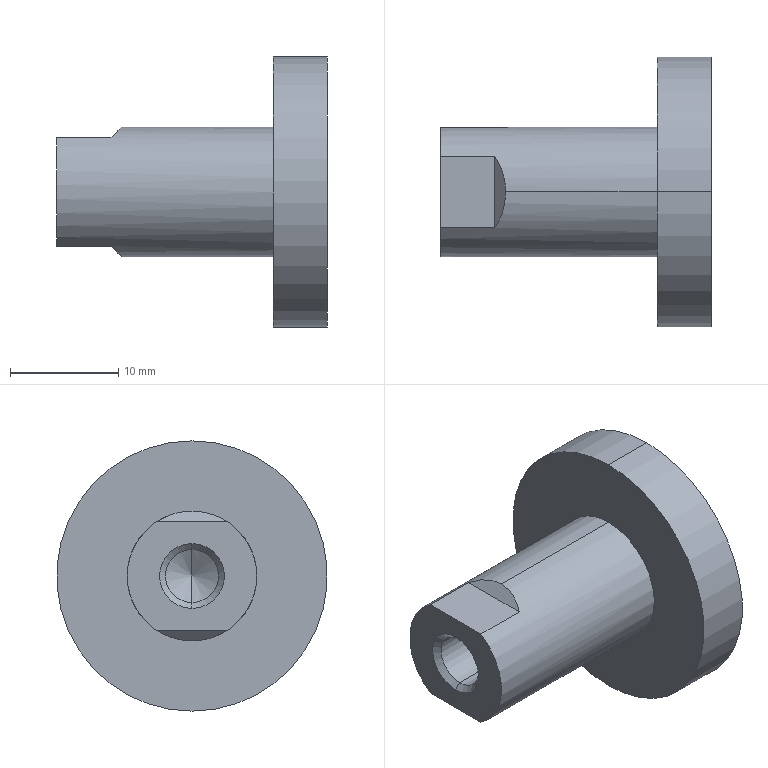Part | STEP file | 2_9 | 1 solid | 17 faces | box 25 x 25 x 25 mm | volume 4428 mm3 | plane 7 | cylinder 6 | cone 4 | commonest cylinder face diameters 4.917 x2 12 x2 25 x2
STEP:
#1=CARTESIAN_POINT('',(0.,0.,0.));
#2=DIRECTION('',(0.,0.,1.));
#3=DIRECTION('',(1.,0.,0.));
#4=AXIS2_PLACEMENT_3D('',#1,#2,#3);
#5=CARTESIAN_POINT('',(15.,0.,-12.5));
#6=VERTEX_POINT('',#5);
#7=CARTESIAN_POINT('',(15.,0.,12.5));
#8=VERTEX_POINT('',#7);
#9=CARTESIAN_POINT('',(15.,0.,0.));
#10=DIRECTION('',(1.,0.,0.));
#11=DIRECTION('',(0.,0.,-1.));
#12=AXIS2_PLACEMENT_3D('',#9,#10,#11);
#13=CIRCLE('',#12,12.5);
#14=CARTESIAN_POINT('',(17.5,0.,0.));
#15=DIRECTION('',(1.,0.,0.));
#16=DIRECTION('',(0.,0.,-1.));
#17=AXIS2_PLACEMENT_3D('',#14,#15,#16);
#18=CYLINDRICAL_SURFACE('',#17,12.5);
#19=CARTESIAN_POINT('',(0.,-2.5));
#20=DIRECTION('',(1.,0.));
#21=VECTOR('',#20,1.);
#22=LINE('',#19,#21);
#23=(GEOMETRIC_REPRESENTATION_CONTEXT(2)PARAMETRIC_REPRESENTATION_CONTEXT()REPRESENTATION_CONTEXT('',''));
#24=DEFINITIONAL_REPRESENTATION('',(#22),#23);
#25=PCURVE('',#18,#24);
#26=CARTESIAN_POINT('',(15.,9.25,0.));
#27=DIRECTION('',(-1.,0.,0.));
#28=DIRECTION('',(0.,0.,1.));
#29=AXIS2_PLACEMENT_3D('',#26,#27,#28);
#30=PLANE('',#29);
#31=CARTESIAN_POINT('',(-12.5,-9.25));
#32=CARTESIAN_POINT('',(-12.5,12.401));
#33=CARTESIAN_POINT('',(6.25,1.575));
#34=CARTESIAN_POINT('',(25.,-9.25));
#35=CARTESIAN_POINT('',(6.25,-20.075));
#36=CARTESIAN_POINT('',(-12.5,-30.901));
#37=CARTESIAN_POINT('',(-12.5,-9.25));
#38=(BOUNDED_CURVE()B_SPLINE_CURVE(2,(#31,#32,#33,#34,#35,#36,#37),.UNSPECIFIED.,.T.,.F.)B_SPLINE_CURVE_WITH_KNOTS((1,2,2,2,2,1),(-2.094,0.,2.094,4.189,6.283,8.378),.UNSPECIFIED.)CURVE()GEOMETRIC_REPRESENTATION_ITEM()RATIONAL_B_SPLINE_CURVE((1.,0.5,1.,0.5,1.,0.5,1.))REPRESENTATION_ITEM(''));
#39=(GEOMETRIC_REPRESENTATION_CONTEXT(2)PARAMETRIC_REPRESENTATION_CONTEXT()REPRESENTATION_CONTEXT('',''));
#40=DEFINITIONAL_REPRESENTATION('',(#38),#39);
#41=PCURVE('',#30,#40);
#42=SURFACE_CURVE('',#13,(#25,#41),.PCURVE_S1.);
#43=EDGE_CURVE('',#6,#8,#42,.T.);
#44=ORIENTED_EDGE('',*,*,#43,.T.);
#45=CARTESIAN_POINT('',(20.,0.,12.5));
#46=VERTEX_POINT('',#45);
#47=CARTESIAN_POINT('',(17.5,0.,12.5));
#48=DIRECTION('',(1.,0.,0.));
#49=VECTOR('',#48,1.);
#50=LINE('',#47,#49);
#51=CARTESIAN_POINT('',(3.142,0.));
#52=DIRECTION('',(0.,1.));
#53=VECTOR('',#52,1.);
#54=LINE('',#51,#53);
#55=(GEOMETRIC_REPRESENTATION_CONTEXT(2)PARAMETRIC_REPRESENTATION_CONTEXT()REPRESENTATION_CONTEXT('',''));
#56=DEFINITIONAL_REPRESENTATION('',(#54),#55);
#57=PCURVE('',#18,#56);
#58=CARTESIAN_POINT('',(17.5,0.,0.));
#59=DIRECTION('',(1.,0.,0.));
#60=DIRECTION('',(0.,0.,-1.));
#61=AXIS2_PLACEMENT_3D('',#58,#59,#60);
#62=CYLINDRICAL_SURFACE('',#61,12.5);
#63=CARTESIAN_POINT('',(3.142,0.));
#64=DIRECTION('',(0.,1.));
#65=VECTOR('',#64,1.);
#66=LINE('',#63,#65);
#67=(GEOMETRIC_REPRESENTATION_CONTEXT(2)PARAMETRIC_REPRESENTATION_CONTEXT()REPRESENTATION_CONTEXT('',''));
#68=DEFINITIONAL_REPRESENTATION('',(#66),#67);
#69=PCURVE('',#62,#68);
#70=SURFACE_CURVE('',#50,(#57,#69),.PCURVE_S1.);
#71=EDGE_CURVE('',#8,#46,#70,.T.);
#72=ORIENTED_EDGE('',*,*,#71,.T.);
#73=CARTESIAN_POINT('',(20.,0.,-12.5));
#74=VERTEX_POINT('',#73);
#75=CARTESIAN_POINT('',(20.,0.,0.));
#76=DIRECTION('',(1.,0.,0.));
#77=DIRECTION('',(0.,0.,-1.));
#78=AXIS2_PLACEMENT_3D('',#75,#76,#77);
#79=CIRCLE('',#78,12.5);
#80=CARTESIAN_POINT('',(0.,2.5));
#81=DIRECTION('',(1.,0.));
#82=VECTOR('',#81,1.);
#83=LINE('',#80,#82);
#84=(GEOMETRIC_REPRESENTATION_CONTEXT(2)PARAMETRIC_REPRESENTATION_CONTEXT()REPRESENTATION_CONTEXT('',''));
#85=DEFINITIONAL_REPRESENTATION('',(#83),#84);
#86=PCURVE('',#18,#85);
#87=CARTESIAN_POINT('',(20.,6.25,0.));
#88=DIRECTION('',(1.,0.,0.));
#89=DIRECTION('',(0.,0.,-1.));
#90=AXIS2_PLACEMENT_3D('',#87,#88,#89);
#91=PLANE('',#90);
#92=CARTESIAN_POINT('',(0.,-6.25));
#93=DIRECTION('',(1.,0.));
#94=AXIS2_PLACEMENT_2D('',#92,#93);
#95=CIRCLE('',#94,12.5);
#96=(GEOMETRIC_REPRESENTATION_CONTEXT(2)PARAMETRIC_REPRESENTATION_CONTEXT()REPRESENTATION_CONTEXT('',''));
#97=DEFINITIONAL_REPRESENTATION('',(#95),#96);
#98=PCURVE('',#91,#97);
#99=SURFACE_CURVE('',#79,(#86,#98),.PCURVE_S1.);
#100=EDGE_CURVE('',#74,#46,#99,.T.);
#101=ORIENTED_EDGE('',*,*,#100,.F.);
#102=CARTESIAN_POINT('',(17.5,0.,-12.5));
#103=DIRECTION('',(1.,0.,0.));
#104=VECTOR('',#103,1.);
#105=LINE('',#102,#104);
#106=CARTESIAN_POINT('',(0.,0.));
#107=DIRECTION('',(0.,1.));
#108=VECTOR('',#107,1.);
#109=LINE('',#106,#108);
#110=(GEOMETRIC_REPRESENTATION_CONTEXT(2)PARAMETRIC_REPRESENTATION_CONTEXT()REPRESENTATION_CONTEXT('',''));
#111=DEFINITIONAL_REPRESENTATION('',(#109),#110);
#112=PCURVE('',#18,#111);
#113=CARTESIAN_POINT('',(6.283,0.));
#114=DIRECTION('',(0.,1.));
#115=VECTOR('',#114,1.);
#116=LINE('',#113,#115);
#117=(GEOMETRIC_REPRESENTATION_CONTEXT(2)PARAMETRIC_REPRESENTATION_CONTEXT()REPRESENTATION_CONTEXT('',''));
#118=DEFINITIONAL_REPRESENTATION('',(#116),#117);
#119=PCURVE('',#62,#118);
#120=SURFACE_CURVE('',#105,(#112,#119),.PCURVE_S1.);
#121=EDGE_CURVE('',#6,#74,#120,.T.);
#122=ORIENTED_EDGE('',*,*,#121,.F.);
#123=EDGE_LOOP('',(#44,#72,#101,#122));
#124=FACE_BOUND('',#123,.T.);
#125=ADVANCED_FACE('',(#124),#18,.T.);
#126=CARTESIAN_POINT('',(0.,3.317,5.));
#127=VERTEX_POINT('',#126);
#128=CARTESIAN_POINT('',(1.,0.,6.));
#129=VERTEX_POINT('',#128);
#130=CARTESIAN_POINT('',(0.,3.317,5.));
#131=CARTESIAN_POINT('',(0.6569,2.326,5.657));
#132=CARTESIAN_POINT('',(1.,1.188,6.));
#133=CARTESIAN_POINT('',(1.,0.,6.));
#134=(BOUNDED_CURVE()B_SPLINE_CURVE(3,(#130,#131,#132,#133),.UNSPECIFIED.,.F.,.F.)B_SPLINE_CURVE_WITH_KNOTS((4,4),(5.697,6.283),.PIECEWISE_BEZIER_KNOTS.)CURVE()GEOMETRIC_REPRESENTATION_ITEM()RATIONAL_B_SPLINE_CURVE((1.,0.9716,0.9716,1.))REPRESENTATION_ITEM(''));
#135=CARTESIAN_POINT('',(5.,0.,0.));
#136=DIRECTION('',(1.,0.,0.));
#137=DIRECTION('',(0.,0.,-1.));
#138=AXIS2_PLACEMENT_3D('',#135,#136,#137);
#139=CYLINDRICAL_SURFACE('',#138,6.);
#140=CARTESIAN_POINT('',(2.556,-5.));
#141=CARTESIAN_POINT('',(2.565,-4.971));
#142=CARTESIAN_POINT('',(2.582,-4.914));
#143=CARTESIAN_POINT('',(2.609,-4.832));
#144=CARTESIAN_POINT('',(2.635,-4.753));
#145=CARTESIAN_POINT('',(2.662,-4.677));
#146=CARTESIAN_POINT('',(2.688,-4.606));
#147=CARTESIAN_POINT('',(2.715,-4.537));
#148=CARTESIAN_POINT('',(2.742,-4.473));
#149=CARTESIAN_POINT('',(2.768,-4.412));
#150=CARTESIAN_POINT('',(2.795,-4.356));
#151=CARTESIAN_POINT('',(2.822,-4.303));
#152=CARTESIAN_POINT('',(2.849,-4.255));
#153=CARTESIAN_POINT('',(2.876,-4.21));
#154=CARTESIAN_POINT('',(2.902,-4.17));
#155=CARTESIAN_POINT('',(2.929,-4.134));
#156=CARTESIAN_POINT('',(2.956,-4.102));
#157=CARTESIAN_POINT('',(2.983,-4.075));
#158=CARTESIAN_POINT('',(3.009,-4.052));
#159=CARTESIAN_POINT('',(3.036,-4.033));
#160=CARTESIAN_POINT('',(3.062,-4.018));
#161=CARTESIAN_POINT('',(3.089,-4.008));
#162=CARTESIAN_POINT('',(3.115,-4.001));
#163=CARTESIAN_POINT('',(3.133,-4.));
#164=CARTESIAN_POINT('',(3.142,-4.));
#165=B_SPLINE_CURVE_WITH_KNOTS('',3,(#140,#141,#142,#143,#144,#145,#146,#147,#148,#149,#150,#151,#152,#153,#154,#155,#156,#157,#158,#159,#160,#161,#162,#163,#164),.UNSPECIFIED.,.F.,.F.,(4,1,1,1,1,1,1,1,1,1,1,1,1,1,1,1,1,1,1,1,1,1,4),(5.697,5.724,5.751,5.777,5.804,5.831,5.857,5.884,5.91,5.937,5.964,5.99,6.017,6.044,6.07,6.097,6.123,6.15,6.177,6.203,6.23,6.257,6.283),.QUASI_UNIFORM_KNOTS.);
#166=(GEOMETRIC_REPRESENTATION_CONTEXT(2)PARAMETRIC_REPRESENTATION_CONTEXT()REPRESENTATION_CONTEXT('',''));
#167=DEFINITIONAL_REPRESENTATION('',(#165),#166);
#168=PCURVE('',#139,#167);
#169=CARTESIAN_POINT('',(5.,12.,10.));
#170=DIRECTION('',(0.7071,0.,-0.7071));
#171=DIRECTION('',(-0.7071,0.,-0.7071));
#172=AXIS2_PLACEMENT_3D('',#169,#170,#171);
#173=PLANE('',#172);
#174=CARTESIAN_POINT('',(7.071,-8.683));
#175=CARTESIAN_POINT('',(6.142,-9.674));
#176=CARTESIAN_POINT('',(5.657,-10.812));
#177=CARTESIAN_POINT('',(5.657,-12.));
#178=(BOUNDED_CURVE()B_SPLINE_CURVE(3,(#174,#175,#176,#177),.UNSPECIFIED.,.F.,.F.)B_SPLINE_CURVE_WITH_KNOTS((4,4),(5.697,6.283),.PIECEWISE_BEZIER_KNOTS.)CURVE()GEOMETRIC_REPRESENTATION_ITEM()RATIONAL_B_SPLINE_CURVE((1.,0.9716,0.9716,1.))REPRESENTATION_ITEM(''));
#179=(GEOMETRIC_REPRESENTATION_CONTEXT(2)PARAMETRIC_REPRESENTATION_CONTEXT()REPRESENTATION_CONTEXT('',''));
#180=DEFINITIONAL_REPRESENTATION('',(#178),#179);
#181=PCURVE('',#173,#180);
#182=SURFACE_CURVE('',#134,(#168,#181),.PCURVE_S1.);
#183=EDGE_CURVE('',#127,#129,#182,.T.);
#184=ORIENTED_EDGE('',*,*,#183,.T.);
#185=CARTESIAN_POINT('',(15.,0.,6.));
#186=VERTEX_POINT('',#185);
#187=CARTESIAN_POINT('',(5.,0.,6.));
#188=DIRECTION('',(1.,0.,0.));
#189=VECTOR('',#188,1.);
#190=LINE('',#187,#189);
#191=CARTESIAN_POINT('',(3.142,0.));
#192=DIRECTION('',(0.,1.));
#193=VECTOR('',#192,1.);
#194=LINE('',#191,#193);
#195=(GEOMETRIC_REPRESENTATION_CONTEXT(2)PARAMETRIC_REPRESENTATION_CONTEXT()REPRESENTATION_CONTEXT('',''));
#196=DEFINITIONAL_REPRESENTATION('',(#194),#195);
#197=PCURVE('',#139,#196);
#198=CARTESIAN_POINT('',(5.,0.,0.));
#199=DIRECTION('',(1.,0.,0.));
#200=DIRECTION('',(0.,0.,-1.));
#201=AXIS2_PLACEMENT_3D('',#198,#199,#200);
#202=CYLINDRICAL_SURFACE('',#201,6.);
#203=CARTESIAN_POINT('',(3.142,0.));
#204=DIRECTION('',(0.,1.));
#205=VECTOR('',#204,1.);
#206=LINE('',#203,#205);
#207=(GEOMETRIC_REPRESENTATION_CONTEXT(2)PARAMETRIC_REPRESENTATION_CONTEXT()REPRESENTATION_CONTEXT('',''));
#208=DEFINITIONAL_REPRESENTATION('',(#206),#207);
#209=PCURVE('',#202,#208);
#210=SURFACE_CURVE('',#190,(#197,#209),.PCURVE_S1.);
#211=EDGE_CURVE('',#129,#186,#210,.T.);
#212=ORIENTED_EDGE('',*,*,#211,.T.);
#213=CARTESIAN_POINT('',(15.,0.,-6.));
#214=VERTEX_POINT('',#213);
#215=CARTESIAN_POINT('',(15.,0.,0.));
#216=DIRECTION('',(1.,0.,0.));
#217=DIRECTION('',(0.,0.,-1.));
#218=AXIS2_PLACEMENT_3D('',#215,#216,#217);
#219=CIRCLE('',#218,6.);
#220=CARTESIAN_POINT('',(0.,10.));
#221=DIRECTION('',(1.,0.));
#222=VECTOR('',#221,1.);
#223=LINE('',#220,#222);
#224=(GEOMETRIC_REPRESENTATION_CONTEXT(2)PARAMETRIC_REPRESENTATION_CONTEXT()REPRESENTATION_CONTEXT('',''));
#225=DEFINITIONAL_REPRESENTATION('',(#223),#224);
#226=PCURVE('',#139,#225);
#227=CARTESIAN_POINT('',(-6.,-9.25));
#228=CARTESIAN_POINT('',(-6.,1.142));
#229=CARTESIAN_POINT('',(3.,-4.054));
#230=CARTESIAN_POINT('',(12.,-9.25));
#231=CARTESIAN_POINT('',(3.,-14.446));
#232=CARTESIAN_POINT('',(-6.,-19.642));
#233=CARTESIAN_POINT('',(-6.,-9.25));
#234=(BOUNDED_CURVE()B_SPLINE_CURVE(2,(#227,#228,#229,#230,#231,#232,#233),.UNSPECIFIED.,.T.,.F.)B_SPLINE_CURVE_WITH_KNOTS((1,2,2,2,2,1),(-2.094,0.,2.094,4.189,6.283,8.378),.UNSPECIFIED.)CURVE()GEOMETRIC_REPRESENTATION_ITEM()RATIONAL_B_SPLINE_CURVE((1.,0.5,1.,0.5,1.,0.5,1.))REPRESENTATION_ITEM(''));
#235=(GEOMETRIC_REPRESENTATION_CONTEXT(2)PARAMETRIC_REPRESENTATION_CONTEXT()REPRESENTATION_CONTEXT('',''));
#236=DEFINITIONAL_REPRESENTATION('',(#234),#235);
#237=PCURVE('',#30,#236);
#238=SURFACE_CURVE('',#219,(#226,#237),.PCURVE_S1.);
#239=EDGE_CURVE('',#214,#186,#238,.T.);
#240=ORIENTED_EDGE('',*,*,#239,.F.);
#241=CARTESIAN_POINT('',(1.,0.,-6.));
#242=VERTEX_POINT('',#241);
#243=CARTESIAN_POINT('',(5.,0.,-6.));
#244=DIRECTION('',(1.,0.,0.));
#245=VECTOR('',#244,1.);
#246=LINE('',#243,#245);
#247=CARTESIAN_POINT('',(0.,0.));
#248=DIRECTION('',(0.,1.));
#249=VECTOR('',#248,1.);
#250=LINE('',#247,#249);
#251=(GEOMETRIC_REPRESENTATION_CONTEXT(2)PARAMETRIC_REPRESENTATION_CONTEXT()REPRESENTATION_CONTEXT('',''));
#252=DEFINITIONAL_REPRESENTATION('',(#250),#251);
#253=PCURVE('',#139,#252);
#254=CARTESIAN_POINT('',(6.283,0.));
#255=DIRECTION('',(0.,1.));
#256=VECTOR('',#255,1.);
#257=LINE('',#254,#256);
#258=(GEOMETRIC_REPRESENTATION_CONTEXT(2)PARAMETRIC_REPRESENTATION_CONTEXT()REPRESENTATION_CONTEXT('',''));
#259=DEFINITIONAL_REPRESENTATION('',(#257),#258);
#260=PCURVE('',#202,#259);
#261=SURFACE_CURVE('',#246,(#253,#260),.PCURVE_S1.);
#262=EDGE_CURVE('',#242,#214,#261,.T.);
#263=ORIENTED_EDGE('',*,*,#262,.F.);
#264=CARTESIAN_POINT('',(0.,3.317,-5.));
#265=VERTEX_POINT('',#264);
#266=CARTESIAN_POINT('',(1.,0.,-6.));
#267=CARTESIAN_POINT('',(1.,1.188,-6.));
#268=CARTESIAN_POINT('',(0.6569,2.326,-5.657));
#269=CARTESIAN_POINT('',(0.,3.317,-5.));
#270=(BOUNDED_CURVE()B_SPLINE_CURVE(3,(#266,#267,#268,#269),.UNSPECIFIED.,.F.,.F.)B_SPLINE_CURVE_WITH_KNOTS((4,4),(0.,0.5857),.PIECEWISE_BEZIER_KNOTS.)CURVE()GEOMETRIC_REPRESENTATION_ITEM()RATIONAL_B_SPLINE_CURVE((1.,0.9716,0.9716,1.))REPRESENTATION_ITEM(''));
#271=CARTESIAN_POINT('',(0.,-4.));
#272=CARTESIAN_POINT('',(0.008748,-4.));
#273=CARTESIAN_POINT('',(0.02628,-4.001));
#274=CARTESIAN_POINT('',(0.05266,-4.008));
#275=CARTESIAN_POINT('',(0.07914,-4.018));
#276=CARTESIAN_POINT('',(0.1057,-4.033));
#277=CARTESIAN_POINT('',(0.1323,-4.052));
#278=CARTESIAN_POINT('',(0.159,-4.075));
#279=CARTESIAN_POINT('',(0.1857,-4.102));
#280=CARTESIAN_POINT('',(0.2124,-4.134));
#281=CARTESIAN_POINT('',(0.2392,-4.17));
#282=CARTESIAN_POINT('',(0.266,-4.21));
#283=CARTESIAN_POINT('',(0.2928,-4.255));
#284=CARTESIAN_POINT('',(0.3197,-4.303));
#285=CARTESIAN_POINT('',(0.3465,-4.356));
#286=CARTESIAN_POINT('',(0.3732,-4.412));
#287=CARTESIAN_POINT('',(0.4,-4.473));
#288=CARTESIAN_POINT('',(0.4267,-4.537));
#289=CARTESIAN_POINT('',(0.4534,-4.606));
#290=CARTESIAN_POINT('',(0.48,-4.677));
#291=CARTESIAN_POINT('',(0.5066,-4.753));
#292=CARTESIAN_POINT('',(0.533,-4.832));
#293=CARTESIAN_POINT('',(0.5594,-4.914));
#294=CARTESIAN_POINT('',(0.5769,-4.971));
#295=CARTESIAN_POINT('',(0.5857,-5.));
#296=B_SPLINE_CURVE_WITH_KNOTS('',3,(#271,#272,#273,#274,#275,#276,#277,#278,#279,#280,#281,#282,#283,#284,#285,#286,#287,#288,#289,#290,#291,#292,#293,#294,#295),.UNSPECIFIED.,.F.,.F.,(4,1,1,1,1,1,1,1,1,1,1,1,1,1,1,1,1,1,1,1,1,1,4),(0.,0.02662,0.05324,0.07987,0.1065,0.1331,0.1597,0.1864,0.213,0.2396,0.2662,0.2928,0.3195,0.3461,0.3727,0.3993,0.426,0.4526,0.4792,0.5058,0.5324,0.5591,0.5857),.QUASI_UNIFORM_KNOTS.);
#297=(GEOMETRIC_REPRESENTATION_CONTEXT(2)PARAMETRIC_REPRESENTATION_CONTEXT()REPRESENTATION_CONTEXT('',''));
#298=DEFINITIONAL_REPRESENTATION('',(#296),#297);
#299=PCURVE('',#139,#298);
#300=CARTESIAN_POINT('',(0.,12.,-5.));
#301=DIRECTION('',(0.7071,0.,0.7071));
#302=DIRECTION('',(0.7071,0.,-0.7071));
#303=AXIS2_PLACEMENT_3D('',#300,#301,#302);
#304=PLANE('',#303);
#305=CARTESIAN_POINT('',(1.414,-12.));
#306=CARTESIAN_POINT('',(1.414,-10.812));
#307=CARTESIAN_POINT('',(0.929,-9.674));
#308=CARTESIAN_POINT('',(0.,-8.683));
#309=(BOUNDED_CURVE()B_SPLINE_CURVE(3,(#305,#306,#307,#308),.UNSPECIFIED.,.F.,.F.)B_SPLINE_CURVE_WITH_KNOTS((4,4),(0.,0.5857),.PIECEWISE_BEZIER_KNOTS.)CURVE()GEOMETRIC_REPRESENTATION_ITEM()RATIONAL_B_SPLINE_CURVE((1.,0.9716,0.9716,1.))REPRESENTATION_ITEM(''));
#310=(GEOMETRIC_REPRESENTATION_CONTEXT(2)PARAMETRIC_REPRESENTATION_CONTEXT()REPRESENTATION_CONTEXT('',''));
#311=DEFINITIONAL_REPRESENTATION('',(#309),#310);
#312=PCURVE('',#304,#311);
#313=SURFACE_CURVE('',#270,(#299,#312),.PCURVE_S1.);
#314=EDGE_CURVE('',#242,#265,#313,.T.);
#315=ORIENTED_EDGE('',*,*,#314,.T.);
#316=CARTESIAN_POINT('',(-5.,3.317,-5.));
#317=VERTEX_POINT('',#316);
#318=CARTESIAN_POINT('',(5.,3.317,-5.));
#319=DIRECTION('',(-1.,0.,0.));
#320=VECTOR('',#319,1.);
#321=LINE('',#318,#320);
#322=CARTESIAN_POINT('',(0.5857,0.));
#323=DIRECTION('',(0.,-1.));
#324=VECTOR('',#323,1.);
#325=LINE('',#322,#324);
#326=(GEOMETRIC_REPRESENTATION_CONTEXT(2)PARAMETRIC_REPRESENTATION_CONTEXT()REPRESENTATION_CONTEXT('',''));
#327=DEFINITIONAL_REPRESENTATION('',(#325),#326);
#328=PCURVE('',#139,#327);
#329=CARTESIAN_POINT('',(-5.,12.,-5.));
#330=DIRECTION('',(0.,0.,1.));
#331=DIRECTION('',(1.,0.,0.));
#332=AXIS2_PLACEMENT_3D('',#329,#330,#331);
#333=PLANE('',#332);
#334=CARTESIAN_POINT('',(10.,-8.683));
#335=DIRECTION('',(-1.,0.));
#336=VECTOR('',#335,1.);
#337=LINE('',#334,#336);
#338=(GEOMETRIC_REPRESENTATION_CONTEXT(2)PARAMETRIC_REPRESENTATION_CONTEXT()REPRESENTATION_CONTEXT('',''));
#339=DEFINITIONAL_REPRESENTATION('',(#337),#338);
#340=PCURVE('',#333,#339);
#341=SURFACE_CURVE('',#321,(#328,#340),.PCURVE_S1.);
#342=EDGE_CURVE('',#265,#317,#341,.T.);
#343=ORIENTED_EDGE('',*,*,#342,.T.);
#344=CARTESIAN_POINT('',(-5.,3.317,5.));
#345=VERTEX_POINT('',#344);
#346=CARTESIAN_POINT('',(-5.,0.,0.));
#347=DIRECTION('',(1.,0.,0.));
#348=DIRECTION('',(0.,0.,-1.));
#349=AXIS2_PLACEMENT_3D('',#346,#347,#348);
#350=CIRCLE('',#349,6.);
#351=CARTESIAN_POINT('',(0.,-10.));
#352=DIRECTION('',(1.,0.));
#353=VECTOR('',#352,1.);
#354=LINE('',#351,#353);
#355=(GEOMETRIC_REPRESENTATION_CONTEXT(2)PARAMETRIC_REPRESENTATION_CONTEXT()REPRESENTATION_CONTEXT('',''));
#356=DEFINITIONAL_REPRESENTATION('',(#354),#355);
#357=PCURVE('',#139,#356);
#358=CARTESIAN_POINT('',(-5.,4.5,0.));
#359=DIRECTION('',(-1.,0.,0.));
#360=DIRECTION('',(0.,0.,1.));
#361=AXIS2_PLACEMENT_3D('',#358,#359,#360);
#362=PLANE('',#361);
#363=CARTESIAN_POINT('',(-6.,-4.5));
#364=CARTESIAN_POINT('',(-6.,5.892));
#365=CARTESIAN_POINT('',(3.,0.6962));
#366=CARTESIAN_POINT('',(12.,-4.5));
#367=CARTESIAN_POINT('',(3.,-9.696));
#368=CARTESIAN_POINT('',(-6.,-14.892));
#369=CARTESIAN_POINT('',(-6.,-4.5));
#370=(BOUNDED_CURVE()B_SPLINE_CURVE(2,(#363,#364,#365,#366,#367,#368,#369),.UNSPECIFIED.,.T.,.F.)B_SPLINE_CURVE_WITH_KNOTS((1,2,2,2,2,1),(-2.094,0.,2.094,4.189,6.283,8.378),.UNSPECIFIED.)CURVE()GEOMETRIC_REPRESENTATION_ITEM()RATIONAL_B_SPLINE_CURVE((1.,0.5,1.,0.5,1.,0.5,1.))REPRESENTATION_ITEM(''));
#371=(GEOMETRIC_REPRESENTATION_CONTEXT(2)PARAMETRIC_REPRESENTATION_CONTEXT()REPRESENTATION_CONTEXT('',''));
#372=DEFINITIONAL_REPRESENTATION('',(#370),#371);
#373=PCURVE('',#362,#372);
#374=SURFACE_CURVE('',#350,(#357,#373),.PCURVE_S1.);
#375=EDGE_CURVE('',#317,#345,#374,.T.);
#376=ORIENTED_EDGE('',*,*,#375,.T.);
#377=CARTESIAN_POINT('',(5.,3.317,5.));
#378=DIRECTION('',(1.,0.,0.));
#379=VECTOR('',#378,1.);
#380=LINE('',#377,#379);
#381=CARTESIAN_POINT('',(2.556,0.));
#382=DIRECTION('',(0.,1.));
#383=VECTOR('',#382,1.);
#384=LINE('',#381,#383);
#385=(GEOMETRIC_REPRESENTATION_CONTEXT(2)PARAMETRIC_REPRESENTATION_CONTEXT()REPRESENTATION_CONTEXT('',''));
#386=DEFINITIONAL_REPRESENTATION('',(#384),#385);
#387=PCURVE('',#139,#386);
#388=CARTESIAN_POINT('',(0.,12.,5.));
#389=DIRECTION('',(0.,0.,-1.));
#390=DIRECTION('',(-1.,0.,0.));
#391=AXIS2_PLACEMENT_3D('',#388,#389,#390);
#392=PLANE('',#391);
#393=CARTESIAN_POINT('',(-5.,-8.683));
#394=DIRECTION('',(-1.,0.));
#395=VECTOR('',#394,1.);
#396=LINE('',#393,#395);
#397=(GEOMETRIC_REPRESENTATION_CONTEXT(2)PARAMETRIC_REPRESENTATION_CONTEXT()REPRESENTATION_CONTEXT('',''));
#398=DEFINITIONAL_REPRESENTATION('',(#396),#397);
#399=PCURVE('',#392,#398);
#400=SURFACE_CURVE('',#380,(#387,#399),.PCURVE_S1.);
#401=EDGE_CURVE('',#345,#127,#400,.T.);
#402=ORIENTED_EDGE('',*,*,#401,.T.);
#403=EDGE_LOOP('',(#184,#212,#240,#263,#315,#343,#376,#402));
#404=FACE_BOUND('',#403,.T.);
#405=ADVANCED_FACE('',(#404),#139,.T.);
#406=CARTESIAN_POINT('',(-4.458,0.,2.458));
#407=VERTEX_POINT('',#406);
#408=CARTESIAN_POINT('',(-5.,0.,3.));
#409=VERTEX_POINT('',#408);
#410=CARTESIAN_POINT('',(-5.,0.,3.));
#411=DIRECTION('',(-0.7071,0.,0.7071));
#412=VECTOR('',#411,1.);
#413=LINE('',#410,#412);
#414=CARTESIAN_POINT('',(-5.,0.,0.));
#415=DIRECTION('',(-1.,0.,0.));
#416=DIRECTION('',(0.,0.,1.));
#417=AXIS2_PLACEMENT_3D('',#414,#415,#416);
#418=CONICAL_SURFACE('',#417,3.,0.7854);
#419=CARTESIAN_POINT('',(6.283,0.));
#420=DIRECTION('',(0.,1.));
#421=VECTOR('',#420,1.);
#422=LINE('',#419,#421);
#423=(GEOMETRIC_REPRESENTATION_CONTEXT(2)PARAMETRIC_REPRESENTATION_CONTEXT()REPRESENTATION_CONTEXT('',''));
#424=DEFINITIONAL_REPRESENTATION('',(#422),#423);
#425=PCURVE('',#418,#424);
#426=CARTESIAN_POINT('',(-5.,0.,0.));
#427=DIRECTION('',(-1.,0.,0.));
#428=DIRECTION('',(0.,0.,1.));
#429=AXIS2_PLACEMENT_3D('',#426,#427,#428);
#430=CONICAL_SURFACE('',#429,3.,0.7854);
#431=CARTESIAN_POINT('',(0.,0.));
#432=DIRECTION('',(0.,1.));
#433=VECTOR('',#432,1.);
#434=LINE('',#431,#433);
#435=(GEOMETRIC_REPRESENTATION_CONTEXT(2)PARAMETRIC_REPRESENTATION_CONTEXT()REPRESENTATION_CONTEXT('',''));
#436=DEFINITIONAL_REPRESENTATION('',(#434),#435);
#437=PCURVE('',#430,#436);
#438=SURFACE_CURVE('',#413,(#425,#437),.PCURVE_S1.);
#439=EDGE_CURVE('',#407,#409,#438,.T.);
#440=ORIENTED_EDGE('',*,*,#439,.T.);
#441=CARTESIAN_POINT('',(-5.,0.,-3.));
#442=VERTEX_POINT('',#441);
#443=CARTESIAN_POINT('',(-5.,0.,0.));
#444=DIRECTION('',(1.,0.,0.));
#445=DIRECTION('',(0.,0.,1.));
#446=AXIS2_PLACEMENT_3D('',#443,#444,#445);
#447=CIRCLE('',#446,3.);
#448=CARTESIAN_POINT('',(6.283,0.));
#449=DIRECTION('',(-1.,0.));
#450=VECTOR('',#449,1.);
#451=LINE('',#448,#450);
#452=(GEOMETRIC_REPRESENTATION_CONTEXT(2)PARAMETRIC_REPRESENTATION_CONTEXT()REPRESENTATION_CONTEXT('',''));
#453=DEFINITIONAL_REPRESENTATION('',(#451),#452);
#454=PCURVE('',#418,#453);
#455=CARTESIAN_POINT('',(3.,-4.5));
#456=CARTESIAN_POINT('',(3.,-9.696));
#457=CARTESIAN_POINT('',(-1.5,-7.098));
#458=CARTESIAN_POINT('',(-6.,-4.5));
#459=CARTESIAN_POINT('',(-1.5,-1.902));
#460=CARTESIAN_POINT('',(3.,0.6962));
#461=CARTESIAN_POINT('',(3.,-4.5));
#462=(BOUNDED_CURVE()B_SPLINE_CURVE(2,(#455,#456,#457,#458,#459,#460,#461),.UNSPECIFIED.,.T.,.F.)B_SPLINE_CURVE_WITH_KNOTS((1,2,2,2,2,1),(-2.094,0.,2.094,4.189,6.283,8.378),.UNSPECIFIED.)CURVE()GEOMETRIC_REPRESENTATION_ITEM()RATIONAL_B_SPLINE_CURVE((1.,0.5,1.,0.5,1.,0.5,1.))REPRESENTATION_ITEM(''));
#463=(GEOMETRIC_REPRESENTATION_CONTEXT(2)PARAMETRIC_REPRESENTATION_CONTEXT()REPRESENTATION_CONTEXT('',''));
#464=DEFINITIONAL_REPRESENTATION('',(#462),#463);
#465=PCURVE('',#362,#464);
#466=SURFACE_CURVE('',#447,(#454,#465),.PCURVE_S1.);
#467=EDGE_CURVE('',#409,#442,#466,.T.);
#468=ORIENTED_EDGE('',*,*,#467,.T.);
#469=CARTESIAN_POINT('',(-4.458,0.,-2.458));
#470=VERTEX_POINT('',#469);
#471=CARTESIAN_POINT('',(-5.,0.,-3.));
#472=DIRECTION('',(-0.7071,0.,-0.7071));
#473=VECTOR('',#472,1.);
#474=LINE('',#471,#473);
#475=CARTESIAN_POINT('',(3.142,0.));
#476=DIRECTION('',(0.,1.));
#477=VECTOR('',#476,1.);
#478=LINE('',#475,#477);
#479=(GEOMETRIC_REPRESENTATION_CONTEXT(2)PARAMETRIC_REPRESENTATION_CONTEXT()REPRESENTATION_CONTEXT('',''));
#480=DEFINITIONAL_REPRESENTATION('',(#478),#479);
#481=PCURVE('',#418,#480);
#482=CARTESIAN_POINT('',(3.142,0.));
#483=DIRECTION('',(0.,1.));
#484=VECTOR('',#483,1.);
#485=LINE('',#482,#484);
#486=(GEOMETRIC_REPRESENTATION_CONTEXT(2)PARAMETRIC_REPRESENTATION_CONTEXT()REPRESENTATION_CONTEXT('',''));
#487=DEFINITIONAL_REPRESENTATION('',(#485),#486);
#488=PCURVE('',#430,#487);
#489=SURFACE_CURVE('',#474,(#481,#488),.PCURVE_S1.);
#490=EDGE_CURVE('',#470,#442,#489,.T.);
#491=ORIENTED_EDGE('',*,*,#490,.F.);
#492=CARTESIAN_POINT('',(-4.458,0.,0.));
#493=DIRECTION('',(-1.,0.,0.));
#494=DIRECTION('',(0.,1.,0.));
#495=AXIS2_PLACEMENT_3D('',#492,#493,#494);
#496=CIRCLE('',#495,2.458);
#497=CARTESIAN_POINT('',(1.571,-0.5415));
#498=DIRECTION('',(1.,0.));
#499=VECTOR('',#498,1.);
#500=LINE('',#497,#499);
#501=(GEOMETRIC_REPRESENTATION_CONTEXT(2)PARAMETRIC_REPRESENTATION_CONTEXT()REPRESENTATION_CONTEXT('',''));
#502=DEFINITIONAL_REPRESENTATION('',(#500),#501);
#503=PCURVE('',#418,#502);
#504=CARTESIAN_POINT('',(1.271,0.,0.));
#505=DIRECTION('',(1.,0.,0.));
#506=DIRECTION('',(0.,0.,-1.));
#507=AXIS2_PLACEMENT_3D('',#504,#505,#506);
#508=CYLINDRICAL_SURFACE('',#507,2.458);
#509=CARTESIAN_POINT('',(7.854,-5.729));
#510=DIRECTION('',(-1.,0.));
#511=VECTOR('',#510,1.);
#512=LINE('',#509,#511);
#513=(GEOMETRIC_REPRESENTATION_CONTEXT(2)PARAMETRIC_REPRESENTATION_CONTEXT()REPRESENTATION_CONTEXT('',''));
#514=DEFINITIONAL_REPRESENTATION('',(#512),#513);
#515=PCURVE('',#508,#514);
#516=SURFACE_CURVE('',#496,(#503,#515),.PCURVE_S1.);
#517=EDGE_CURVE('',#470,#407,#516,.T.);
#518=ORIENTED_EDGE('',*,*,#517,.T.);
#519=EDGE_LOOP('',(#440,#468,#491,#518));
#520=FACE_BOUND('',#519,.F.);
#521=ADVANCED_FACE('',(#520),#418,.F.);
#522=CARTESIAN_POINT('',(7.,0.,-2.458));
#523=VERTEX_POINT('',#522);
#524=CARTESIAN_POINT('',(1.271,0.,-2.458));
#525=DIRECTION('',(1.,0.,0.));
#526=VECTOR('',#525,1.);
#527=LINE('',#524,#526);
#528=CARTESIAN_POINT('',(6.283,0.));
#529=DIRECTION('',(0.,1.));
#530=VECTOR('',#529,1.);
#531=LINE('',#528,#530);
#532=(GEOMETRIC_REPRESENTATION_CONTEXT(2)PARAMETRIC_REPRESENTATION_CONTEXT()REPRESENTATION_CONTEXT('',''));
#533=DEFINITIONAL_REPRESENTATION('',(#531),#532);
#534=PCURVE('',#508,#533);
#535=CARTESIAN_POINT('',(1.271,0.,0.));
#536=DIRECTION('',(1.,0.,0.));
#537=DIRECTION('',(0.,0.,-1.));
#538=AXIS2_PLACEMENT_3D('',#535,#536,#537);
#539=CYLINDRICAL_SURFACE('',#538,2.458);
#540=CARTESIAN_POINT('',(0.,0.));
#541=DIRECTION('',(0.,1.));
#542=VECTOR('',#541,1.);
#543=LINE('',#540,#542);
#544=(GEOMETRIC_REPRESENTATION_CONTEXT(2)PARAMETRIC_REPRESENTATION_CONTEXT()REPRESENTATION_CONTEXT('',''));
#545=DEFINITIONAL_REPRESENTATION('',(#543),#544);
#546=PCURVE('',#539,#545);
#547=SURFACE_CURVE('',#527,(#534,#546),.PCURVE_S1.);
#548=EDGE_CURVE('',#470,#523,#547,.T.);
#549=ORIENTED_EDGE('',*,*,#548,.T.);
#550=CARTESIAN_POINT('',(7.,0.,2.458));
#551=VERTEX_POINT('',#550);
#552=CARTESIAN_POINT('',(7.,0.,0.));
#553=DIRECTION('',(-1.,0.,0.));
#554=DIRECTION('',(0.,0.,-1.));
#555=AXIS2_PLACEMENT_3D('',#552,#553,#554);
#556=CIRCLE('',#555,2.458);
#557=CARTESIAN_POINT('',(6.283,5.729));
#558=DIRECTION('',(-1.,0.));
#559=VECTOR('',#558,1.);
#560=LINE('',#557,#559);
#561=(GEOMETRIC_REPRESENTATION_CONTEXT(2)PARAMETRIC_REPRESENTATION_CONTEXT()REPRESENTATION_CONTEXT('',''));
#562=DEFINITIONAL_REPRESENTATION('',(#560),#561);
#563=PCURVE('',#508,#562);
#564=CARTESIAN_POINT('',(7.,0.,0.));
#565=DIRECTION('',(-1.,0.,0.));
#566=DIRECTION('',(0.,0.,1.));
#567=AXIS2_PLACEMENT_3D('',#564,#565,#566);
#568=CONICAL_SURFACE('',#567,2.458,1.047);
#569=CARTESIAN_POINT('',(3.142,0.));
#570=DIRECTION('',(1.,0.));
#571=VECTOR('',#570,1.);
#572=LINE('',#569,#571);
#573=(GEOMETRIC_REPRESENTATION_CONTEXT(2)PARAMETRIC_REPRESENTATION_CONTEXT()REPRESENTATION_CONTEXT('',''));
#574=DEFINITIONAL_REPRESENTATION('',(#572),#573);
#575=PCURVE('',#568,#574);
#576=SURFACE_CURVE('',#556,(#563,#575),.PCURVE_S1.);
#577=EDGE_CURVE('',#523,#551,#576,.T.);
#578=ORIENTED_EDGE('',*,*,#577,.T.);
#579=CARTESIAN_POINT('',(1.271,0.,2.458));
#580=DIRECTION('',(1.,0.,0.));
#581=VECTOR('',#580,1.);
#582=LINE('',#579,#581);
#583=CARTESIAN_POINT('',(3.142,0.));
#584=DIRECTION('',(0.,1.));
#585=VECTOR('',#584,1.);
#586=LINE('',#583,#585);
#587=(GEOMETRIC_REPRESENTATION_CONTEXT(2)PARAMETRIC_REPRESENTATION_CONTEXT()REPRESENTATION_CONTEXT('',''));
#588=DEFINITIONAL_REPRESENTATION('',(#586),#587);
#589=PCURVE('',#508,#588);
#590=CARTESIAN_POINT('',(3.142,0.));
#591=DIRECTION('',(0.,1.));
#592=VECTOR('',#591,1.);
#593=LINE('',#590,#592);
#594=(GEOMETRIC_REPRESENTATION_CONTEXT(2)PARAMETRIC_REPRESENTATION_CONTEXT()REPRESENTATION_CONTEXT('',''));
#595=DEFINITIONAL_REPRESENTATION('',(#593),#594);
#596=PCURVE('',#539,#595);
#597=SURFACE_CURVE('',#582,(#589,#596),.PCURVE_S1.);
#598=EDGE_CURVE('',#407,#551,#597,.T.);
#599=ORIENTED_EDGE('',*,*,#598,.F.);
#600=ORIENTED_EDGE('',*,*,#517,.F.);
#601=EDGE_LOOP('',(#549,#578,#599,#600));
#602=FACE_BOUND('',#601,.F.);
#603=ADVANCED_FACE('',(#602),#508,.F.);
#604=ORIENTED_EDGE('',*,*,#577,.F.);
#605=CARTESIAN_POINT('',(8.419,0.,0.));
#606=VERTEX_POINT('',#605);
#607=CARTESIAN_POINT('',(7.,0.,-2.458));
#608=DIRECTION('',(-0.5,0.,-0.866));
#609=VECTOR('',#608,1.);
#610=LINE('',#607,#609);
#611=CARTESIAN_POINT('',(3.142,0.));
#612=DIRECTION('',(0.,1.));
#613=VECTOR('',#612,1.);
#614=LINE('',#611,#613);
#615=(GEOMETRIC_REPRESENTATION_CONTEXT(2)PARAMETRIC_REPRESENTATION_CONTEXT()REPRESENTATION_CONTEXT('',''));
#616=DEFINITIONAL_REPRESENTATION('',(#614),#615);
#617=PCURVE('',#568,#616);
#618=CARTESIAN_POINT('',(7.,0.,0.));
#619=DIRECTION('',(-1.,0.,0.));
#620=DIRECTION('',(0.,0.,1.));
#621=AXIS2_PLACEMENT_3D('',#618,#619,#620);
#622=CONICAL_SURFACE('',#621,2.458,1.047);
#623=CARTESIAN_POINT('',(3.142,0.));
#624=DIRECTION('',(0.,1.));
#625=VECTOR('',#624,1.);
#626=LINE('',#623,#625);
#627=(GEOMETRIC_REPRESENTATION_CONTEXT(2)PARAMETRIC_REPRESENTATION_CONTEXT()REPRESENTATION_CONTEXT('',''));
#628=DEFINITIONAL_REPRESENTATION('',(#626),#627);
#629=PCURVE('',#622,#628);
#630=SURFACE_CURVE('',#610,(#617,#629),.PCURVE_S1.);
#631=EDGE_CURVE('',#606,#523,#630,.T.);
#632=ORIENTED_EDGE('',*,*,#631,.F.);
#633=CARTESIAN_POINT('',(7.,0.,2.458));
#634=DIRECTION('',(-0.5,0.,0.866));
#635=VECTOR('',#634,1.);
#636=LINE('',#633,#635);
#637=CARTESIAN_POINT('',(6.283,0.));
#638=DIRECTION('',(0.,1.));
#639=VECTOR('',#638,1.);
#640=LINE('',#637,#639);
#641=(GEOMETRIC_REPRESENTATION_CONTEXT(2)PARAMETRIC_REPRESENTATION_CONTEXT()REPRESENTATION_CONTEXT('',''));
#642=DEFINITIONAL_REPRESENTATION('',(#640),#641);
#643=PCURVE('',#568,#642);
#644=CARTESIAN_POINT('',(0.,0.));
#645=DIRECTION('',(0.,1.));
#646=VECTOR('',#645,1.);
#647=LINE('',#644,#646);
#648=(GEOMETRIC_REPRESENTATION_CONTEXT(2)PARAMETRIC_REPRESENTATION_CONTEXT()REPRESENTATION_CONTEXT('',''));
#649=DEFINITIONAL_REPRESENTATION('',(#647),#648);
#650=PCURVE('',#622,#649);
#651=SURFACE_CURVE('',#636,(#643,#650),.PCURVE_S1.);
#652=EDGE_CURVE('',#606,#551,#651,.T.);
#653=ORIENTED_EDGE('',*,*,#652,.T.);
#654=EDGE_LOOP('',(#604,#632,#653));
#655=FACE_BOUND('',#654,.F.);
#656=ADVANCED_FACE('',(#655),#568,.F.);
#657=ORIENTED_EDGE('',*,*,#100,.T.);
#658=CARTESIAN_POINT('',(20.,0.,0.));
#659=DIRECTION('',(1.,0.,0.));
#660=DIRECTION('',(0.,0.,-1.));
#661=AXIS2_PLACEMENT_3D('',#658,#659,#660);
#662=CIRCLE('',#661,12.5);
#663=CARTESIAN_POINT('',(0.,-6.25));
#664=DIRECTION('',(1.,0.));
#665=AXIS2_PLACEMENT_2D('',#663,#664);
#666=CIRCLE('',#665,12.5);
#667=(GEOMETRIC_REPRESENTATION_CONTEXT(2)PARAMETRIC_REPRESENTATION_CONTEXT()REPRESENTATION_CONTEXT('',''));
#668=DEFINITIONAL_REPRESENTATION('',(#666),#667);
#669=PCURVE('',#91,#668);
#670=CARTESIAN_POINT('',(0.,2.5));
#671=DIRECTION('',(1.,0.));
#672=VECTOR('',#671,1.);
#673=LINE('',#670,#672);
#674=(GEOMETRIC_REPRESENTATION_CONTEXT(2)PARAMETRIC_REPRESENTATION_CONTEXT()REPRESENTATION_CONTEXT('',''));
#675=DEFINITIONAL_REPRESENTATION('',(#673),#674);
#676=PCURVE('',#62,#675);
#677=SURFACE_CURVE('',#662,(#669,#676),.PCURVE_S1.);
#678=EDGE_CURVE('',#46,#74,#677,.T.);
#679=ORIENTED_EDGE('',*,*,#678,.T.);
#680=EDGE_LOOP('',(#657,#679));
#681=FACE_BOUND('',#680,.T.);
#682=ADVANCED_FACE('',(#681),#91,.T.);
#683=ORIENTED_EDGE('',*,*,#71,.F.);
#684=CARTESIAN_POINT('',(15.,0.,0.));
#685=DIRECTION('',(1.,0.,0.));
#686=DIRECTION('',(0.,0.,-1.));
#687=AXIS2_PLACEMENT_3D('',#684,#685,#686);
#688=CIRCLE('',#687,12.5);
#689=CARTESIAN_POINT('',(0.,-2.5));
#690=DIRECTION('',(1.,0.));
#691=VECTOR('',#690,1.);
#692=LINE('',#689,#691);
#693=(GEOMETRIC_REPRESENTATION_CONTEXT(2)PARAMETRIC_REPRESENTATION_CONTEXT()REPRESENTATION_CONTEXT('',''));
#694=DEFINITIONAL_REPRESENTATION('',(#692),#693);
#695=PCURVE('',#62,#694);
#696=CARTESIAN_POINT('',(-12.5,-9.25));
#697=CARTESIAN_POINT('',(-12.5,12.401));
#698=CARTESIAN_POINT('',(6.25,1.575));
#699=CARTESIAN_POINT('',(25.,-9.25));
#700=CARTESIAN_POINT('',(6.25,-20.075));
#701=CARTESIAN_POINT('',(-12.5,-30.901));
#702=CARTESIAN_POINT('',(-12.5,-9.25));
#703=(BOUNDED_CURVE()B_SPLINE_CURVE(2,(#696,#697,#698,#699,#700,#701,#702),.UNSPECIFIED.,.T.,.F.)B_SPLINE_CURVE_WITH_KNOTS((1,2,2,2,2,1),(-2.094,0.,2.094,4.189,6.283,8.378),.UNSPECIFIED.)CURVE()GEOMETRIC_REPRESENTATION_ITEM()RATIONAL_B_SPLINE_CURVE((1.,0.5,1.,0.5,1.,0.5,1.))REPRESENTATION_ITEM(''));
#704=(GEOMETRIC_REPRESENTATION_CONTEXT(2)PARAMETRIC_REPRESENTATION_CONTEXT()REPRESENTATION_CONTEXT('',''));
#705=DEFINITIONAL_REPRESENTATION('',(#703),#704);
#706=PCURVE('',#30,#705);
#707=SURFACE_CURVE('',#688,(#695,#706),.PCURVE_S1.);
#708=EDGE_CURVE('',#8,#6,#707,.T.);
#709=ORIENTED_EDGE('',*,*,#708,.T.);
#710=ORIENTED_EDGE('',*,*,#121,.T.);
#711=ORIENTED_EDGE('',*,*,#678,.F.);
#712=EDGE_LOOP('',(#683,#709,#710,#711));
#713=FACE_BOUND('',#712,.T.);
#714=ADVANCED_FACE('',(#713),#62,.T.);
#715=ORIENTED_EDGE('',*,*,#43,.F.);
#716=ORIENTED_EDGE('',*,*,#708,.F.);
#717=EDGE_LOOP('',(#715,#716));
#718=FACE_BOUND('',#717,.T.);
#719=ORIENTED_EDGE('',*,*,#239,.T.);
#720=CARTESIAN_POINT('',(15.,0.,0.));
#721=DIRECTION('',(1.,0.,0.));
#722=DIRECTION('',(0.,0.,-1.));
#723=AXIS2_PLACEMENT_3D('',#720,#721,#722);
#724=CIRCLE('',#723,6.);
#725=CARTESIAN_POINT('',(-6.,-9.25));
#726=CARTESIAN_POINT('',(-6.,1.142));
#727=CARTESIAN_POINT('',(3.,-4.054));
#728=CARTESIAN_POINT('',(12.,-9.25));
#729=CARTESIAN_POINT('',(3.,-14.446));
#730=CARTESIAN_POINT('',(-6.,-19.642));
#731=CARTESIAN_POINT('',(-6.,-9.25));
#732=(BOUNDED_CURVE()B_SPLINE_CURVE(2,(#725,#726,#727,#728,#729,#730,#731),.UNSPECIFIED.,.T.,.F.)B_SPLINE_CURVE_WITH_KNOTS((1,2,2,2,2,1),(-2.094,0.,2.094,4.189,6.283,8.378),.UNSPECIFIED.)CURVE()GEOMETRIC_REPRESENTATION_ITEM()RATIONAL_B_SPLINE_CURVE((1.,0.5,1.,0.5,1.,0.5,1.))REPRESENTATION_ITEM(''));
#733=(GEOMETRIC_REPRESENTATION_CONTEXT(2)PARAMETRIC_REPRESENTATION_CONTEXT()REPRESENTATION_CONTEXT('',''));
#734=DEFINITIONAL_REPRESENTATION('',(#732),#733);
#735=PCURVE('',#30,#734);
#736=CARTESIAN_POINT('',(0.,10.));
#737=DIRECTION('',(1.,0.));
#738=VECTOR('',#737,1.);
#739=LINE('',#736,#738);
#740=(GEOMETRIC_REPRESENTATION_CONTEXT(2)PARAMETRIC_REPRESENTATION_CONTEXT()REPRESENTATION_CONTEXT('',''));
#741=DEFINITIONAL_REPRESENTATION('',(#739),#740);
#742=PCURVE('',#202,#741);
#743=SURFACE_CURVE('',#724,(#735,#742),.PCURVE_S1.);
#744=EDGE_CURVE('',#186,#214,#743,.T.);
#745=ORIENTED_EDGE('',*,*,#744,.T.);
#746=EDGE_LOOP('',(#719,#745));
#747=FACE_BOUND('',#746,.T.);
#748=ADVANCED_FACE('',(#718,#747),#30,.T.);
#749=ORIENTED_EDGE('',*,*,#211,.F.);
#750=CARTESIAN_POINT('',(0.,-3.317,5.));
#751=VERTEX_POINT('',#750);
#752=CARTESIAN_POINT('',(1.,0.,6.));
#753=CARTESIAN_POINT('',(1.,-1.188,6.));
#754=CARTESIAN_POINT('',(0.6569,-2.326,5.657));
#755=CARTESIAN_POINT('',(0.,-3.317,5.));
#756=(BOUNDED_CURVE()B_SPLINE_CURVE(3,(#752,#753,#754,#755),.UNSPECIFIED.,.F.,.F.)B_SPLINE_CURVE_WITH_KNOTS((4,4),(0.,0.5857),.PIECEWISE_BEZIER_KNOTS.)CURVE()GEOMETRIC_REPRESENTATION_ITEM()RATIONAL_B_SPLINE_CURVE((1.,0.9716,0.9716,1.))REPRESENTATION_ITEM(''));
#757=CARTESIAN_POINT('',(3.142,-4.));
#758=CARTESIAN_POINT('',(3.15,-4.));
#759=CARTESIAN_POINT('',(3.168,-4.001));
#760=CARTESIAN_POINT('',(3.194,-4.008));
#761=CARTESIAN_POINT('',(3.221,-4.018));
#762=CARTESIAN_POINT('',(3.247,-4.033));
#763=CARTESIAN_POINT('',(3.274,-4.052));
#764=CARTESIAN_POINT('',(3.301,-4.075));
#765=CARTESIAN_POINT('',(3.327,-4.102));
#766=CARTESIAN_POINT('',(3.354,-4.134));
#767=CARTESIAN_POINT('',(3.381,-4.17));
#768=CARTESIAN_POINT('',(3.408,-4.21));
#769=CARTESIAN_POINT('',(3.434,-4.255));
#770=CARTESIAN_POINT('',(3.461,-4.303));
#771=CARTESIAN_POINT('',(3.488,-4.356));
#772=CARTESIAN_POINT('',(3.515,-4.412));
#773=CARTESIAN_POINT('',(3.542,-4.473));
#774=CARTESIAN_POINT('',(3.568,-4.537));
#775=CARTESIAN_POINT('',(3.595,-4.606));
#776=CARTESIAN_POINT('',(3.622,-4.677));
#777=CARTESIAN_POINT('',(3.648,-4.753));
#778=CARTESIAN_POINT('',(3.675,-4.832));
#779=CARTESIAN_POINT('',(3.701,-4.914));
#780=CARTESIAN_POINT('',(3.719,-4.971));
#781=CARTESIAN_POINT('',(3.727,-5.));
#782=B_SPLINE_CURVE_WITH_KNOTS('',3,(#757,#758,#759,#760,#761,#762,#763,#764,#765,#766,#767,#768,#769,#770,#771,#772,#773,#774,#775,#776,#777,#778,#779,#780,#781),.UNSPECIFIED.,.F.,.F.,(4,1,1,1,1,1,1,1,1,1,1,1,1,1,1,1,1,1,1,1,1,1,4),(0.,0.02662,0.05324,0.07987,0.1065,0.1331,0.1597,0.1864,0.213,0.2396,0.2662,0.2928,0.3195,0.3461,0.3727,0.3993,0.426,0.4526,0.4792,0.5058,0.5324,0.5591,0.5857),.QUASI_UNIFORM_KNOTS.);
#783=(GEOMETRIC_REPRESENTATION_CONTEXT(2)PARAMETRIC_REPRESENTATION_CONTEXT()REPRESENTATION_CONTEXT('',''));
#784=DEFINITIONAL_REPRESENTATION('',(#782),#783);
#785=PCURVE('',#202,#784);
#786=CARTESIAN_POINT('',(5.657,-12.));
#787=CARTESIAN_POINT('',(5.657,-13.188));
#788=CARTESIAN_POINT('',(6.142,-14.326));
#789=CARTESIAN_POINT('',(7.071,-15.317));
#790=(BOUNDED_CURVE()B_SPLINE_CURVE(3,(#786,#787,#788,#789),.UNSPECIFIED.,.F.,.F.)B_SPLINE_CURVE_WITH_KNOTS((4,4),(0.,0.5857),.PIECEWISE_BEZIER_KNOTS.)CURVE()GEOMETRIC_REPRESENTATION_ITEM()RATIONAL_B_SPLINE_CURVE((1.,0.9716,0.9716,1.))REPRESENTATION_ITEM(''));
#791=(GEOMETRIC_REPRESENTATION_CONTEXT(2)PARAMETRIC_REPRESENTATION_CONTEXT()REPRESENTATION_CONTEXT('',''));
#792=DEFINITIONAL_REPRESENTATION('',(#790),#791);
#793=PCURVE('',#173,#792);
#794=SURFACE_CURVE('',#756,(#785,#793),.PCURVE_S1.);
#795=EDGE_CURVE('',#129,#751,#794,.T.);
#796=ORIENTED_EDGE('',*,*,#795,.T.);
#797=CARTESIAN_POINT('',(-5.,-3.317,5.));
#798=VERTEX_POINT('',#797);
#799=CARTESIAN_POINT('',(5.,-3.317,5.));
#800=DIRECTION('',(-1.,0.,0.));
#801=VECTOR('',#800,1.);
#802=LINE('',#799,#801);
#803=CARTESIAN_POINT('',(3.727,0.));
#804=DIRECTION('',(0.,-1.));
#805=VECTOR('',#804,1.);
#806=LINE('',#803,#805);
#807=(GEOMETRIC_REPRESENTATION_CONTEXT(2)PARAMETRIC_REPRESENTATION_CONTEXT()REPRESENTATION_CONTEXT('',''));
#808=DEFINITIONAL_REPRESENTATION('',(#806),#807);
#809=PCURVE('',#202,#808);
#810=CARTESIAN_POINT('',(-5.,-15.317));
#811=DIRECTION('',(1.,0.));
#812=VECTOR('',#811,1.);
#813=LINE('',#810,#812);
#814=(GEOMETRIC_REPRESENTATION_CONTEXT(2)PARAMETRIC_REPRESENTATION_CONTEXT()REPRESENTATION_CONTEXT('',''));
#815=DEFINITIONAL_REPRESENTATION('',(#813),#814);
#816=PCURVE('',#392,#815);
#817=SURFACE_CURVE('',#802,(#809,#816),.PCURVE_S1.);
#818=EDGE_CURVE('',#751,#798,#817,.T.);
#819=ORIENTED_EDGE('',*,*,#818,.T.);
#820=CARTESIAN_POINT('',(-5.,-3.317,-5.));
#821=VERTEX_POINT('',#820);
#822=CARTESIAN_POINT('',(-5.,0.,0.));
#823=DIRECTION('',(1.,0.,0.));
#824=DIRECTION('',(0.,0.,-1.));
#825=AXIS2_PLACEMENT_3D('',#822,#823,#824);
#826=CIRCLE('',#825,6.);
#827=CARTESIAN_POINT('',(0.,-10.));
#828=DIRECTION('',(1.,0.));
#829=VECTOR('',#828,1.);
#830=LINE('',#827,#829);
#831=(GEOMETRIC_REPRESENTATION_CONTEXT(2)PARAMETRIC_REPRESENTATION_CONTEXT()REPRESENTATION_CONTEXT('',''));
#832=DEFINITIONAL_REPRESENTATION('',(#830),#831);
#833=PCURVE('',#202,#832);
#834=CARTESIAN_POINT('',(-6.,-4.5));
#835=CARTESIAN_POINT('',(-6.,5.892));
#836=CARTESIAN_POINT('',(3.,0.6962));
#837=CARTESIAN_POINT('',(12.,-4.5));
#838=CARTESIAN_POINT('',(3.,-9.696));
#839=CARTESIAN_POINT('',(-6.,-14.892));
#840=CARTESIAN_POINT('',(-6.,-4.5));
#841=(BOUNDED_CURVE()B_SPLINE_CURVE(2,(#834,#835,#836,#837,#838,#839,#840),.UNSPECIFIED.,.T.,.F.)B_SPLINE_CURVE_WITH_KNOTS((1,2,2,2,2,1),(-2.094,0.,2.094,4.189,6.283,8.378),.UNSPECIFIED.)CURVE()GEOMETRIC_REPRESENTATION_ITEM()RATIONAL_B_SPLINE_CURVE((1.,0.5,1.,0.5,1.,0.5,1.))REPRESENTATION_ITEM(''));
#842=(GEOMETRIC_REPRESENTATION_CONTEXT(2)PARAMETRIC_REPRESENTATION_CONTEXT()REPRESENTATION_CONTEXT('',''));
#843=DEFINITIONAL_REPRESENTATION('',(#841),#842);
#844=PCURVE('',#362,#843);
#845=SURFACE_CURVE('',#826,(#833,#844),.PCURVE_S1.);
#846=EDGE_CURVE('',#798,#821,#845,.T.);
#847=ORIENTED_EDGE('',*,*,#846,.T.);
#848=CARTESIAN_POINT('',(0.,-3.317,-5.));
#849=VERTEX_POINT('',#848);
#850=CARTESIAN_POINT('',(5.,-3.317,-5.));
#851=DIRECTION('',(1.,0.,0.));
#852=VECTOR('',#851,1.);
#853=LINE('',#850,#852);
#854=CARTESIAN_POINT('',(5.697,0.));
#855=DIRECTION('',(0.,1.));
#856=VECTOR('',#855,1.);
#857=LINE('',#854,#856);
#858=(GEOMETRIC_REPRESENTATION_CONTEXT(2)PARAMETRIC_REPRESENTATION_CONTEXT()REPRESENTATION_CONTEXT('',''));
#859=DEFINITIONAL_REPRESENTATION('',(#857),#858);
#860=PCURVE('',#202,#859);
#861=CARTESIAN_POINT('',(10.,-15.317));
#862=DIRECTION('',(1.,0.));
#863=VECTOR('',#862,1.);
#864=LINE('',#861,#863);
#865=(GEOMETRIC_REPRESENTATION_CONTEXT(2)PARAMETRIC_REPRESENTATION_CONTEXT()REPRESENTATION_CONTEXT('',''));
#866=DEFINITIONAL_REPRESENTATION('',(#864),#865);
#867=PCURVE('',#333,#866);
#868=SURFACE_CURVE('',#853,(#860,#867),.PCURVE_S1.);
#869=EDGE_CURVE('',#821,#849,#868,.T.);
#870=ORIENTED_EDGE('',*,*,#869,.T.);
#871=CARTESIAN_POINT('',(0.,-3.317,-5.));
#872=CARTESIAN_POINT('',(0.6569,-2.326,-5.657));
#873=CARTESIAN_POINT('',(1.,-1.188,-6.));
#874=CARTESIAN_POINT('',(1.,0.,-6.));
#875=(BOUNDED_CURVE()B_SPLINE_CURVE(3,(#871,#872,#873,#874),.UNSPECIFIED.,.F.,.F.)B_SPLINE_CURVE_WITH_KNOTS((4,4),(5.697,6.283),.PIECEWISE_BEZIER_KNOTS.)CURVE()GEOMETRIC_REPRESENTATION_ITEM()RATIONAL_B_SPLINE_CURVE((1.,0.9716,0.9716,1.))REPRESENTATION_ITEM(''));
#876=CARTESIAN_POINT('',(5.697,-5.));
#877=CARTESIAN_POINT('',(5.706,-4.971));
#878=CARTESIAN_POINT('',(5.724,-4.914));
#879=CARTESIAN_POINT('',(5.75,-4.832));
#880=CARTESIAN_POINT('',(5.777,-4.753));
#881=CARTESIAN_POINT('',(5.803,-4.677));
#882=CARTESIAN_POINT('',(5.83,-4.606));
#883=CARTESIAN_POINT('',(5.856,-4.537));
#884=CARTESIAN_POINT('',(5.883,-4.473));
#885=CARTESIAN_POINT('',(5.91,-4.412));
#886=CARTESIAN_POINT('',(5.937,-4.356));
#887=CARTESIAN_POINT('',(5.964,-4.303));
#888=CARTESIAN_POINT('',(5.99,-4.255));
#889=CARTESIAN_POINT('',(6.017,-4.21));
#890=CARTESIAN_POINT('',(6.044,-4.17));
#891=CARTESIAN_POINT('',(6.071,-4.134));
#892=CARTESIAN_POINT('',(6.098,-4.102));
#893=CARTESIAN_POINT('',(6.124,-4.075));
#894=CARTESIAN_POINT('',(6.151,-4.052));
#895=CARTESIAN_POINT('',(6.178,-4.033));
#896=CARTESIAN_POINT('',(6.204,-4.018));
#897=CARTESIAN_POINT('',(6.231,-4.008));
#898=CARTESIAN_POINT('',(6.257,-4.001));
#899=CARTESIAN_POINT('',(6.274,-4.));
#900=CARTESIAN_POINT('',(6.283,-4.));
#901=B_SPLINE_CURVE_WITH_KNOTS('',3,(#876,#877,#878,#879,#880,#881,#882,#883,#884,#885,#886,#887,#888,#889,#890,#891,#892,#893,#894,#895,#896,#897,#898,#899,#900),.UNSPECIFIED.,.F.,.F.,(4,1,1,1,1,1,1,1,1,1,1,1,1,1,1,1,1,1,1,1,1,1,4),(5.697,5.724,5.751,5.777,5.804,5.831,5.857,5.884,5.91,5.937,5.964,5.99,6.017,6.044,6.07,6.097,6.123,6.15,6.177,6.203,6.23,6.257,6.283),.QUASI_UNIFORM_KNOTS.);
#902=(GEOMETRIC_REPRESENTATION_CONTEXT(2)PARAMETRIC_REPRESENTATION_CONTEXT()REPRESENTATION_CONTEXT('',''));
#903=DEFINITIONAL_REPRESENTATION('',(#901),#902);
#904=PCURVE('',#202,#903);
#905=CARTESIAN_POINT('',(0.,-15.317));
#906=CARTESIAN_POINT('',(0.929,-14.326));
#907=CARTESIAN_POINT('',(1.414,-13.188));
#908=CARTESIAN_POINT('',(1.414,-12.));
#909=(BOUNDED_CURVE()B_SPLINE_CURVE(3,(#905,#906,#907,#908),.UNSPECIFIED.,.F.,.F.)B_SPLINE_CURVE_WITH_KNOTS((4,4),(5.697,6.283),.PIECEWISE_BEZIER_KNOTS.)CURVE()GEOMETRIC_REPRESENTATION_ITEM()RATIONAL_B_SPLINE_CURVE((1.,0.9716,0.9716,1.))REPRESENTATION_ITEM(''));
#910=(GEOMETRIC_REPRESENTATION_CONTEXT(2)PARAMETRIC_REPRESENTATION_CONTEXT()REPRESENTATION_CONTEXT('',''));
#911=DEFINITIONAL_REPRESENTATION('',(#909),#910);
#912=PCURVE('',#304,#911);
#913=SURFACE_CURVE('',#875,(#904,#912),.PCURVE_S1.);
#914=EDGE_CURVE('',#849,#242,#913,.T.);
#915=ORIENTED_EDGE('',*,*,#914,.T.);
#916=ORIENTED_EDGE('',*,*,#262,.T.);
#917=ORIENTED_EDGE('',*,*,#744,.F.);
#918=EDGE_LOOP('',(#749,#796,#819,#847,#870,#915,#916,#917));
#919=FACE_BOUND('',#918,.T.);
#920=ADVANCED_FACE('',(#919),#202,.T.);
#921=CARTESIAN_POINT('',(-5.,4.5,-5.));
#922=DIRECTION('',(0.,-1.,0.));
#923=VECTOR('',#922,1.);
#924=LINE('',#921,#923);
#925=CARTESIAN_POINT('',(-5.,0.));
#926=DIRECTION('',(0.,-1.));
#927=VECTOR('',#926,1.);
#928=LINE('',#925,#927);
#929=(GEOMETRIC_REPRESENTATION_CONTEXT(2)PARAMETRIC_REPRESENTATION_CONTEXT()REPRESENTATION_CONTEXT('',''));
#930=DEFINITIONAL_REPRESENTATION('',(#928),#929);
#931=PCURVE('',#362,#930);
#932=CARTESIAN_POINT('',(0.,-7.5));
#933=DIRECTION('',(0.,-1.));
#934=VECTOR('',#933,1.);
#935=LINE('',#932,#934);
#936=(GEOMETRIC_REPRESENTATION_CONTEXT(2)PARAMETRIC_REPRESENTATION_CONTEXT()REPRESENTATION_CONTEXT('',''));
#937=DEFINITIONAL_REPRESENTATION('',(#935),#936);
#938=PCURVE('',#333,#937);
#939=SURFACE_CURVE('',#924,(#931,#938),.PCURVE_S1.);
#940=EDGE_CURVE('',#317,#821,#939,.T.);
#941=ORIENTED_EDGE('',*,*,#940,.T.);
#942=ORIENTED_EDGE('',*,*,#846,.F.);
#943=CARTESIAN_POINT('',(-5.,4.5,5.));
#944=DIRECTION('',(0.,1.,0.));
#945=VECTOR('',#944,1.);
#946=LINE('',#943,#945);
#947=CARTESIAN_POINT('',(5.,0.));
#948=DIRECTION('',(0.,1.));
#949=VECTOR('',#948,1.);
#950=LINE('',#947,#949);
#951=(GEOMETRIC_REPRESENTATION_CONTEXT(2)PARAMETRIC_REPRESENTATION_CONTEXT()REPRESENTATION_CONTEXT('',''));
#952=DEFINITIONAL_REPRESENTATION('',(#950),#951);
#953=PCURVE('',#362,#952);
#954=CARTESIAN_POINT('',(5.,-7.5));
#955=DIRECTION('',(0.,1.));
#956=VECTOR('',#955,1.);
#957=LINE('',#954,#956);
#958=(GEOMETRIC_REPRESENTATION_CONTEXT(2)PARAMETRIC_REPRESENTATION_CONTEXT()REPRESENTATION_CONTEXT('',''));
#959=DEFINITIONAL_REPRESENTATION('',(#957),#958);
#960=PCURVE('',#392,#959);
#961=SURFACE_CURVE('',#946,(#953,#960),.PCURVE_S1.);
#962=EDGE_CURVE('',#798,#345,#961,.T.);
#963=ORIENTED_EDGE('',*,*,#962,.T.);
#964=ORIENTED_EDGE('',*,*,#375,.F.);
#965=EDGE_LOOP('',(#941,#942,#963,#964));
#966=FACE_BOUND('',#965,.T.);
#967=ORIENTED_EDGE('',*,*,#467,.T.);
#968=CARTESIAN_POINT('',(-5.,0.,0.));
#969=DIRECTION('',(1.,0.,0.));
#970=DIRECTION('',(0.,0.,1.));
#971=AXIS2_PLACEMENT_3D('',#968,#969,#970);
#972=CIRCLE('',#971,3.);
#973=CARTESIAN_POINT('',(3.,-4.5));
#974=CARTESIAN_POINT('',(3.,-9.696));
#975=CARTESIAN_POINT('',(-1.5,-7.098));
#976=CARTESIAN_POINT('',(-6.,-4.5));
#977=CARTESIAN_POINT('',(-1.5,-1.902));
#978=CARTESIAN_POINT('',(3.,0.6962));
#979=CARTESIAN_POINT('',(3.,-4.5));
#980=(BOUNDED_CURVE()B_SPLINE_CURVE(2,(#973,#974,#975,#976,#977,#978,#979),.UNSPECIFIED.,.T.,.F.)B_SPLINE_CURVE_WITH_KNOTS((1,2,2,2,2,1),(-2.094,0.,2.094,4.189,6.283,8.378),.UNSPECIFIED.)CURVE()GEOMETRIC_REPRESENTATION_ITEM()RATIONAL_B_SPLINE_CURVE((1.,0.5,1.,0.5,1.,0.5,1.))REPRESENTATION_ITEM(''));
#981=(GEOMETRIC_REPRESENTATION_CONTEXT(2)PARAMETRIC_REPRESENTATION_CONTEXT()REPRESENTATION_CONTEXT('',''));
#982=DEFINITIONAL_REPRESENTATION('',(#980),#981);
#983=PCURVE('',#362,#982);
#984=CARTESIAN_POINT('',(6.283,0.));
#985=DIRECTION('',(-1.,0.));
#986=VECTOR('',#985,1.);
#987=LINE('',#984,#986);
#988=(GEOMETRIC_REPRESENTATION_CONTEXT(2)PARAMETRIC_REPRESENTATION_CONTEXT()REPRESENTATION_CONTEXT('',''));
#989=DEFINITIONAL_REPRESENTATION('',(#987),#988);
#990=PCURVE('',#430,#989);
#991=SURFACE_CURVE('',#972,(#983,#990),.PCURVE_S1.);
#992=EDGE_CURVE('',#442,#409,#991,.T.);
#993=ORIENTED_EDGE('',*,*,#992,.T.);
#994=EDGE_LOOP('',(#967,#993));
#995=FACE_BOUND('',#994,.T.);
#996=ADVANCED_FACE('',(#966,#995),#362,.T.);
#997=CARTESIAN_POINT('',(0.,12.,5.));
#998=DIRECTION('',(0.,-1.,0.));
#999=VECTOR('',#998,1.);
#1000=LINE('',#997,#999);
#1001=CARTESIAN_POINT('',(0.,0.));
#1002=DIRECTION('',(0.,-1.));
#1003=VECTOR('',#1002,1.);
#1004=LINE('',#1001,#1003);
#1005=(GEOMETRIC_REPRESENTATION_CONTEXT(2)PARAMETRIC_REPRESENTATION_CONTEXT()REPRESENTATION_CONTEXT('',''));
#1006=DEFINITIONAL_REPRESENTATION('',(#1004),#1005);
#1007=PCURVE('',#392,#1006);
#1008=CARTESIAN_POINT('',(7.071,0.));
#1009=DIRECTION('',(0.,-1.));
#1010=VECTOR('',#1009,1.);
#1011=LINE('',#1008,#1010);
#1012=(GEOMETRIC_REPRESENTATION_CONTEXT(2)PARAMETRIC_REPRESENTATION_CONTEXT()REPRESENTATION_CONTEXT('',''));
#1013=DEFINITIONAL_REPRESENTATION('',(#1011),#1012);
#1014=PCURVE('',#173,#1013);
#1015=SURFACE_CURVE('',#1000,(#1007,#1014),.PCURVE_S1.);
#1016=EDGE_CURVE('',#127,#751,#1015,.T.);
#1017=ORIENTED_EDGE('',*,*,#1016,.F.);
#1018=ORIENTED_EDGE('',*,*,#401,.F.);
#1019=ORIENTED_EDGE('',*,*,#962,.F.);
#1020=ORIENTED_EDGE('',*,*,#818,.F.);
#1021=EDGE_LOOP('',(#1017,#1018,#1019,#1020));
#1022=FACE_BOUND('',#1021,.T.);
#1023=ADVANCED_FACE('',(#1022),#392,.F.);
#1024=ORIENTED_EDGE('',*,*,#1016,.T.);
#1025=ORIENTED_EDGE('',*,*,#795,.F.);
#1026=ORIENTED_EDGE('',*,*,#183,.F.);
#1027=EDGE_LOOP('',(#1024,#1025,#1026));
#1028=FACE_BOUND('',#1027,.T.);
#1029=ADVANCED_FACE('',(#1028),#173,.F.);
#1030=ORIENTED_EDGE('',*,*,#940,.F.);
#1031=ORIENTED_EDGE('',*,*,#342,.F.);
#1032=CARTESIAN_POINT('',(0.,12.,-5.));
#1033=DIRECTION('',(0.,1.,0.));
#1034=VECTOR('',#1033,1.);
#1035=LINE('',#1032,#1034);
#1036=CARTESIAN_POINT('',(5.,0.));
#1037=DIRECTION('',(0.,1.));
#1038=VECTOR('',#1037,1.);
#1039=LINE('',#1036,#1038);
#1040=(GEOMETRIC_REPRESENTATION_CONTEXT(2)PARAMETRIC_REPRESENTATION_CONTEXT()REPRESENTATION_CONTEXT('',''));
#1041=DEFINITIONAL_REPRESENTATION('',(#1039),#1040);
#1042=PCURVE('',#333,#1041);
#1043=CARTESIAN_POINT('',(0.,0.));
#1044=DIRECTION('',(0.,1.));
#1045=VECTOR('',#1044,1.);
#1046=LINE('',#1043,#1045);
#1047=(GEOMETRIC_REPRESENTATION_CONTEXT(2)PARAMETRIC_REPRESENTATION_CONTEXT()REPRESENTATION_CONTEXT('',''));
#1048=DEFINITIONAL_REPRESENTATION('',(#1046),#1047);
#1049=PCURVE('',#304,#1048);
#1050=SURFACE_CURVE('',#1035,(#1042,#1049),.PCURVE_S1.);
#1051=EDGE_CURVE('',#849,#265,#1050,.T.);
#1052=ORIENTED_EDGE('',*,*,#1051,.F.);
#1053=ORIENTED_EDGE('',*,*,#869,.F.);
#1054=EDGE_LOOP('',(#1030,#1031,#1052,#1053));
#1055=FACE_BOUND('',#1054,.T.);
#1056=ADVANCED_FACE('',(#1055),#333,.F.);
#1057=ORIENTED_EDGE('',*,*,#1051,.T.);
#1058=ORIENTED_EDGE('',*,*,#314,.F.);
#1059=ORIENTED_EDGE('',*,*,#914,.F.);
#1060=EDGE_LOOP('',(#1057,#1058,#1059));
#1061=FACE_BOUND('',#1060,.T.);
#1062=ADVANCED_FACE('',(#1061),#304,.F.);
#1063=ORIENTED_EDGE('',*,*,#992,.T.);
#1064=ORIENTED_EDGE('',*,*,#439,.F.);
#1065=CARTESIAN_POINT('',(-4.458,0.,0.));
#1066=DIRECTION('',(-1.,0.,0.));
#1067=DIRECTION('',(0.,1.,0.));
#1068=AXIS2_PLACEMENT_3D('',#1065,#1066,#1067);
#1069=CIRCLE('',#1068,2.458);
#1070=CARTESIAN_POINT('',(-4.712,-0.5415));
#1071=DIRECTION('',(1.,0.));
#1072=VECTOR('',#1071,1.);
#1073=LINE('',#1070,#1072);
#1074=(GEOMETRIC_REPRESENTATION_CONTEXT(2)PARAMETRIC_REPRESENTATION_CONTEXT()REPRESENTATION_CONTEXT('',''));
#1075=DEFINITIONAL_REPRESENTATION('',(#1073),#1074);
#1076=PCURVE('',#430,#1075);
#1077=CARTESIAN_POINT('',(7.854,-5.729));
#1078=DIRECTION('',(-1.,0.));
#1079=VECTOR('',#1078,1.);
#1080=LINE('',#1077,#1079);
#1081=(GEOMETRIC_REPRESENTATION_CONTEXT(2)PARAMETRIC_REPRESENTATION_CONTEXT()REPRESENTATION_CONTEXT('',''));
#1082=DEFINITIONAL_REPRESENTATION('',(#1080),#1081);
#1083=PCURVE('',#539,#1082);
#1084=SURFACE_CURVE('',#1069,(#1076,#1083),.PCURVE_S1.);
#1085=EDGE_CURVE('',#407,#470,#1084,.T.);
#1086=ORIENTED_EDGE('',*,*,#1085,.T.);
#1087=ORIENTED_EDGE('',*,*,#490,.T.);
#1088=EDGE_LOOP('',(#1063,#1064,#1086,#1087));
#1089=FACE_BOUND('',#1088,.F.);
#1090=ADVANCED_FACE('',(#1089),#430,.F.);
#1091=CARTESIAN_POINT('',(7.,0.,0.));
#1092=DIRECTION('',(-1.,0.,0.));
#1093=DIRECTION('',(0.,0.,-1.));
#1094=AXIS2_PLACEMENT_3D('',#1091,#1092,#1093);
#1095=CIRCLE('',#1094,2.458);
#1096=CARTESIAN_POINT('',(6.283,5.729));
#1097=DIRECTION('',(-1.,0.));
#1098=VECTOR('',#1097,1.);
#1099=LINE('',#1096,#1098);
#1100=(GEOMETRIC_REPRESENTATION_CONTEXT(2)PARAMETRIC_REPRESENTATION_CONTEXT()REPRESENTATION_CONTEXT('',''));
#1101=DEFINITIONAL_REPRESENTATION('',(#1099),#1100);
#1102=PCURVE('',#539,#1101);
#1103=CARTESIAN_POINT('',(-3.142,0.));
#1104=DIRECTION('',(1.,0.));
#1105=VECTOR('',#1104,1.);
#1106=LINE('',#1103,#1105);
#1107=(GEOMETRIC_REPRESENTATION_CONTEXT(2)PARAMETRIC_REPRESENTATION_CONTEXT()REPRESENTATION_CONTEXT('',''));
#1108=DEFINITIONAL_REPRESENTATION('',(#1106),#1107);
#1109=PCURVE('',#622,#1108);
#1110=SURFACE_CURVE('',#1095,(#1102,#1109),.PCURVE_S1.);
#1111=EDGE_CURVE('',#551,#523,#1110,.T.);
#1112=ORIENTED_EDGE('',*,*,#1111,.T.);
#1113=ORIENTED_EDGE('',*,*,#548,.F.);
#1114=ORIENTED_EDGE('',*,*,#1085,.F.);
#1115=ORIENTED_EDGE('',*,*,#598,.T.);
#1116=EDGE_LOOP('',(#1112,#1113,#1114,#1115));
#1117=FACE_BOUND('',#1116,.F.);
#1118=ADVANCED_FACE('',(#1117),#539,.F.);
#1119=ORIENTED_EDGE('',*,*,#1111,.F.);
#1120=ORIENTED_EDGE('',*,*,#652,.F.);
#1121=ORIENTED_EDGE('',*,*,#631,.T.);
#1122=EDGE_LOOP('',(#1119,#1120,#1121));
#1123=FACE_BOUND('',#1122,.F.);
#1124=ADVANCED_FACE('',(#1123),#622,.F.);
#1125=CLOSED_SHELL('',(#125,#405,#521,#603,#656,#682,#714,#748,#920,#996,#1023,#1029,#1056,#1062,#1090,#1118,#1124));
#1126=MANIFOLD_SOLID_BREP('',#1125);
#1127=(LENGTH_UNIT()NAMED_UNIT(*)SI_UNIT(.MILLI.,.METRE.));
#1128=UNCERTAINTY_MEASURE_WITH_UNIT(LENGTH_MEASURE(0.0000001),#1127,'','');
#1129=(NAMED_UNIT(*)PLANE_ANGLE_UNIT()SI_UNIT($,.RADIAN.));
#1130=(NAMED_UNIT(*)SI_UNIT($,.STERADIAN.)SOLID_ANGLE_UNIT());
#1131=(GEOMETRIC_REPRESENTATION_CONTEXT(3)GLOBAL_UNCERTAINTY_ASSIGNED_CONTEXT((#1128))GLOBAL_UNIT_ASSIGNED_CONTEXT((#1127,#1129,#1130))REPRESENTATION_CONTEXT('',''));
#1132=ADVANCED_BREP_SHAPE_REPRESENTATION('',(#4,#1126),#1131);